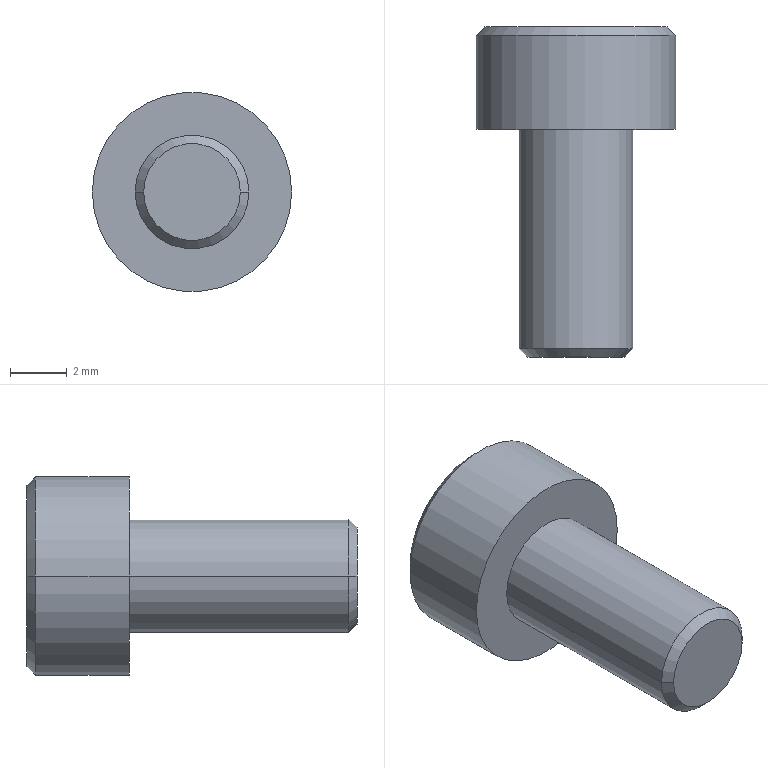Part | NX | 1 solid | 56 faces | box 7 x 11.6 x 7 mm | volume 221.628 mm3 | plane 44 | cone 6 | cylinder 6 | commonest cylinder face diameters 3 x2 4 x2 7 x2
STEP:
#1=CARTESIAN_POINT('',(-1.7,-8.,0.));
#2=VERTEX_POINT('',#1);
#3=CARTESIAN_POINT('',(1.7,-8.,0.));
#4=VERTEX_POINT('',#3);
#5=CARTESIAN_POINT('',(0.,-8.,0.));
#6=DIRECTION('',(0.,1.,0.));
#7=DIRECTION('',(-1.,0.,0.));
#8=AXIS2_PLACEMENT_3D('',#5,#6,#7);
#9=CIRCLE('',#8,1.7);
#10=EDGE_CURVE('',#2,#4,#9,.T.);
#11=ORIENTED_EDGE('',*,*,#10,.F.);
#12=CARTESIAN_POINT('',(0.,-8.,0.));
#13=DIRECTION('',(0.,1.,0.));
#14=DIRECTION('',(-1.,0.,0.));
#15=AXIS2_PLACEMENT_3D('',#12,#13,#14);
#16=CIRCLE('',#15,1.7);
#17=EDGE_CURVE('',#4,#2,#16,.T.);
#18=ORIENTED_EDGE('',*,*,#17,.F.);
#19=EDGE_LOOP('',(#11,#18));
#20=FACE_BOUND('',#19,.T.);
#21=CARTESIAN_POINT('',(0.,-8.,0.));
#22=DIRECTION('',(0.,-1.,0.));
#23=DIRECTION('',(0.,0.,-1.));
#24=AXIS2_PLACEMENT_3D('',#21,#22,#23);
#25=PLANE('',#24);
#26=ADVANCED_FACE('',(#20),#25,.T.);
#27=ORIENTED_EDGE('',*,*,#10,.T.);
#28=CARTESIAN_POINT('',(2.,-7.7,0.));
#29=VERTEX_POINT('',#28);
#30=CARTESIAN_POINT('',(1.85,-7.85,0.));
#31=DIRECTION('',(0.7071,0.7071,0.));
#32=VECTOR('',#31,1000.);
#33=LINE('',#30,#32);
#34=EDGE_CURVE('',#4,#29,#33,.T.);
#35=ORIENTED_EDGE('',*,*,#34,.T.);
#36=CARTESIAN_POINT('',(-2.,-7.7,0.));
#37=VERTEX_POINT('',#36);
#38=CARTESIAN_POINT('',(0.,-7.7,0.));
#39=DIRECTION('',(0.,1.,0.));
#40=DIRECTION('',(-1.,0.,0.));
#41=AXIS2_PLACEMENT_3D('',#38,#39,#40);
#42=CIRCLE('',#41,2.);
#43=EDGE_CURVE('',#37,#29,#42,.T.);
#44=ORIENTED_EDGE('',*,*,#43,.F.);
#45=CARTESIAN_POINT('',(-1.85,-7.85,0.));
#46=DIRECTION('',(-0.7071,0.7071,0.));
#47=VECTOR('',#46,1000.);
#48=LINE('',#45,#47);
#49=EDGE_CURVE('',#2,#37,#48,.T.);
#50=ORIENTED_EDGE('',*,*,#49,.F.);
#51=EDGE_LOOP('',(#27,#35,#44,#50));
#52=FACE_BOUND('',#51,.T.);
#53=CARTESIAN_POINT('',(0.,-7.85,0.));
#54=DIRECTION('',(0.,1.,0.));
#55=DIRECTION('',(1.,0.,0.));
#56=AXIS2_PLACEMENT_3D('',#53,#54,#55);
#57=CONICAL_SURFACE('',#56,1.85,0.7854);
#58=ADVANCED_FACE('',(#52),#57,.T.);
#59=CARTESIAN_POINT('',(0.,-7.7,0.));
#60=DIRECTION('',(0.,1.,0.));
#61=DIRECTION('',(-1.,0.,0.));
#62=AXIS2_PLACEMENT_3D('',#59,#60,#61);
#63=CIRCLE('',#62,2.);
#64=EDGE_CURVE('',#29,#37,#63,.T.);
#65=ORIENTED_EDGE('',*,*,#64,.T.);
#66=CARTESIAN_POINT('',(-2.,0.,0.));
#67=VERTEX_POINT('',#66);
#68=CARTESIAN_POINT('',(-2.,4.18,0.));
#69=DIRECTION('',(0.,-1.,0.));
#70=VECTOR('',#69,1000.);
#71=LINE('',#68,#70);
#72=EDGE_CURVE('',#37,#67,#71,.F.);
#73=ORIENTED_EDGE('',*,*,#72,.T.);
#74=CARTESIAN_POINT('',(2.,0.,0.));
#75=VERTEX_POINT('',#74);
#76=CARTESIAN_POINT('',(0.,0.,0.));
#77=DIRECTION('',(0.,-1.,0.));
#78=DIRECTION('',(1.,0.,0.));
#79=AXIS2_PLACEMENT_3D('',#76,#77,#78);
#80=CIRCLE('',#79,2.);
#81=EDGE_CURVE('',#67,#75,#80,.T.);
#82=ORIENTED_EDGE('',*,*,#81,.T.);
#83=CARTESIAN_POINT('',(2.,4.18,0.));
#84=DIRECTION('',(0.,-1.,0.));
#85=VECTOR('',#84,1000.);
#86=LINE('',#83,#85);
#87=EDGE_CURVE('',#29,#75,#86,.F.);
#88=ORIENTED_EDGE('',*,*,#87,.F.);
#89=EDGE_LOOP('',(#65,#73,#82,#88));
#90=FACE_BOUND('',#89,.T.);
#91=CARTESIAN_POINT('',(0.,4.18,0.));
#92=DIRECTION('',(0.,-1.,0.));
#93=DIRECTION('',(-1.,0.,0.));
#94=AXIS2_PLACEMENT_3D('',#91,#92,#93);
#95=CYLINDRICAL_SURFACE('',#94,2.);
#96=ADVANCED_FACE('',(#90),#95,.T.);
#97=CARTESIAN_POINT('',(0.1875,3.6,1.945));
#98=VERTEX_POINT('',#97);
#99=CARTESIAN_POINT('',(0.4,3.6,1.702));
#100=VERTEX_POINT('',#99);
#101=CARTESIAN_POINT('',(0.1875,3.6,1.945));
#102=DIRECTION('',(0.659,0.,-0.7522));
#103=VECTOR('',#102,1000.);
#104=LINE('',#101,#103);
#105=EDGE_CURVE('',#98,#100,#104,.T.);
#106=ORIENTED_EDGE('',*,*,#105,.F.);
#107=CARTESIAN_POINT('',(0.4,3.6,1.945));
#108=VERTEX_POINT('',#107);
#109=CARTESIAN_POINT('',(0.1875,3.6,1.945));
#110=DIRECTION('',(1.,0.,0.));
#111=VECTOR('',#110,1000.);
#112=LINE('',#109,#111);
#113=EDGE_CURVE('',#98,#108,#112,.T.);
#114=ORIENTED_EDGE('',*,*,#113,.T.);
#115=CARTESIAN_POINT('',(0.4,3.6,1.945));
#116=DIRECTION('',(0.,0.,-1.));
#117=VECTOR('',#116,1000.);
#118=LINE('',#115,#117);
#119=EDGE_CURVE('',#108,#100,#118,.T.);
#120=ORIENTED_EDGE('',*,*,#119,.T.);
#121=EDGE_LOOP('',(#106,#114,#120));
#122=FACE_BOUND('',#121,.T.);
#123=CARTESIAN_POINT('',(0.,3.6,0.));
#124=DIRECTION('',(0.,-1.,0.));
#125=DIRECTION('',(0.,0.,-1.));
#126=AXIS2_PLACEMENT_3D('',#123,#124,#125);
#127=PLANE('',#126);
#128=ADVANCED_FACE('',(#122),#127,.F.);
#129=CARTESIAN_POINT('',(0.1,3.55,1.945));
#130=VERTEX_POINT('',#129);
#131=CARTESIAN_POINT('',(0.4,3.55,1.6));
#132=VERTEX_POINT('',#131);
#133=CARTESIAN_POINT('',(0.1,3.55,1.945));
#134=DIRECTION('',(0.6565,0.,-0.7543));
#135=VECTOR('',#134,1000.);
#136=LINE('',#133,#135);
#137=EDGE_CURVE('',#130,#132,#136,.T.);
#138=ORIENTED_EDGE('',*,*,#137,.F.);
#139=CARTESIAN_POINT('',(0.1,3.55,2.021));
#140=VERTEX_POINT('',#139);
#141=CARTESIAN_POINT('',(0.1,3.55,2.021));
#142=DIRECTION('',(0.,0.,-1.));
#143=VECTOR('',#142,1000.);
#144=LINE('',#141,#143);
#145=EDGE_CURVE('',#140,#130,#144,.T.);
#146=ORIENTED_EDGE('',*,*,#145,.F.);
#147=CARTESIAN_POINT('',(0.4,3.55,2.021));
#148=VERTEX_POINT('',#147);
#149=CARTESIAN_POINT('',(0.4,3.55,2.021));
#150=DIRECTION('',(-1.,0.,0.));
#151=VECTOR('',#150,1000.);
#152=LINE('',#149,#151);
#153=EDGE_CURVE('',#148,#140,#152,.T.);
#154=ORIENTED_EDGE('',*,*,#153,.F.);
#155=CARTESIAN_POINT('',(0.4,3.55,2.2));
#156=VERTEX_POINT('',#155);
#157=CARTESIAN_POINT('',(0.4,3.55,2.2));
#158=DIRECTION('',(0.,0.,-1.));
#159=VECTOR('',#158,1000.);
#160=LINE('',#157,#159);
#161=EDGE_CURVE('',#156,#148,#160,.T.);
#162=ORIENTED_EDGE('',*,*,#161,.F.);
#163=CARTESIAN_POINT('',(0.475,3.55,2.2));
#164=VERTEX_POINT('',#163);
#165=CARTESIAN_POINT('',(0.475,3.55,2.2));
#166=DIRECTION('',(-1.,0.,0.));
#167=VECTOR('',#166,1000.);
#168=LINE('',#165,#167);
#169=EDGE_CURVE('',#164,#156,#168,.T.);
#170=ORIENTED_EDGE('',*,*,#169,.F.);
#171=CARTESIAN_POINT('',(0.475,3.55,2.021));
#172=VERTEX_POINT('',#171);
#173=CARTESIAN_POINT('',(0.475,3.55,2.021));
#174=DIRECTION('',(0.,0.,1.));
#175=VECTOR('',#174,1000.);
#176=LINE('',#173,#175);
#177=EDGE_CURVE('',#172,#164,#176,.T.);
#178=ORIENTED_EDGE('',*,*,#177,.F.);
#179=CARTESIAN_POINT('',(0.6,3.55,2.021));
#180=VERTEX_POINT('',#179);
#181=CARTESIAN_POINT('',(0.6,3.55,2.021));
#182=DIRECTION('',(-1.,0.,0.));
#183=VECTOR('',#182,1000.);
#184=LINE('',#181,#183);
#185=EDGE_CURVE('',#180,#172,#184,.T.);
#186=ORIENTED_EDGE('',*,*,#185,.F.);
#187=CARTESIAN_POINT('',(0.6,3.55,1.945));
#188=VERTEX_POINT('',#187);
#189=CARTESIAN_POINT('',(0.6,3.55,1.945));
#190=DIRECTION('',(0.,0.,1.));
#191=VECTOR('',#190,1000.);
#192=LINE('',#189,#191);
#193=EDGE_CURVE('',#188,#180,#192,.T.);
#194=ORIENTED_EDGE('',*,*,#193,.F.);
#195=CARTESIAN_POINT('',(0.475,3.55,1.945));
#196=VERTEX_POINT('',#195);
#197=CARTESIAN_POINT('',(0.475,3.55,1.945));
#198=DIRECTION('',(1.,0.,0.));
#199=VECTOR('',#198,1000.);
#200=LINE('',#197,#199);
#201=EDGE_CURVE('',#196,#188,#200,.T.);
#202=ORIENTED_EDGE('',*,*,#201,.F.);
#203=CARTESIAN_POINT('',(0.475,3.55,1.6));
#204=VERTEX_POINT('',#203);
#205=CARTESIAN_POINT('',(0.475,3.55,1.6));
#206=DIRECTION('',(0.,0.,1.));
#207=VECTOR('',#206,1000.);
#208=LINE('',#205,#207);
#209=EDGE_CURVE('',#204,#196,#208,.T.);
#210=ORIENTED_EDGE('',*,*,#209,.F.);
#211=CARTESIAN_POINT('',(0.4,3.55,1.6));
#212=DIRECTION('',(1.,0.,0.));
#213=VECTOR('',#212,1000.);
#214=LINE('',#211,#213);
#215=EDGE_CURVE('',#132,#204,#214,.T.);
#216=ORIENTED_EDGE('',*,*,#215,.F.);
#217=EDGE_LOOP('',(#138,#146,#154,#162,#170,#178,#186,#194,#202,#210,#216));
#218=FACE_BOUND('',#217,.T.);
#219=CARTESIAN_POINT('',(0.4,3.55,1.702));
#220=VERTEX_POINT('',#219);
#221=CARTESIAN_POINT('',(0.1875,3.55,1.945));
#222=VERTEX_POINT('',#221);
#223=CARTESIAN_POINT('',(0.4,3.55,1.702));
#224=DIRECTION('',(-0.659,0.,0.7522));
#225=VECTOR('',#224,1000.);
#226=LINE('',#223,#225);
#227=EDGE_CURVE('',#220,#222,#226,.T.);
#228=ORIENTED_EDGE('',*,*,#227,.F.);
#229=CARTESIAN_POINT('',(0.4,3.55,1.945));
#230=VERTEX_POINT('',#229);
#231=CARTESIAN_POINT('',(0.4,3.55,1.945));
#232=DIRECTION('',(0.,0.,-1.));
#233=VECTOR('',#232,1000.);
#234=LINE('',#231,#233);
#235=EDGE_CURVE('',#230,#220,#234,.T.);
#236=ORIENTED_EDGE('',*,*,#235,.F.);
#237=CARTESIAN_POINT('',(0.1875,3.55,1.945));
#238=DIRECTION('',(1.,0.,0.));
#239=VECTOR('',#238,1000.);
#240=LINE('',#237,#239);
#241=EDGE_CURVE('',#222,#230,#240,.T.);
#242=ORIENTED_EDGE('',*,*,#241,.F.);
#243=EDGE_LOOP('',(#228,#236,#242));
#244=FACE_BOUND('',#243,.T.);
#245=CARTESIAN_POINT('',(0.,3.55,0.));
#246=DIRECTION('',(0.,1.,0.));
#247=DIRECTION('',(1.,0.,0.));
#248=AXIS2_PLACEMENT_3D('',#245,#246,#247);
#249=PLANE('',#248);
#250=ADVANCED_FACE('',(#218,#244),#249,.T.);
#251=CARTESIAN_POINT('',(3.5,0.,0.));
#252=VERTEX_POINT('',#251);
#253=CARTESIAN_POINT('',(-3.5,0.,0.));
#254=VERTEX_POINT('',#253);
#255=CARTESIAN_POINT('',(0.,0.,0.));
#256=DIRECTION('',(0.,1.,0.));
#257=DIRECTION('',(-1.,0.,0.));
#258=AXIS2_PLACEMENT_3D('',#255,#256,#257);
#259=CIRCLE('',#258,3.5);
#260=EDGE_CURVE('',#252,#254,#259,.T.);
#261=ORIENTED_EDGE('',*,*,#260,.F.);
#262=CARTESIAN_POINT('',(0.,0.,0.));
#263=DIRECTION('',(0.,1.,0.));
#264=DIRECTION('',(-1.,0.,0.));
#265=AXIS2_PLACEMENT_3D('',#262,#263,#264);
#266=CIRCLE('',#265,3.5);
#267=EDGE_CURVE('',#254,#252,#266,.T.);
#268=ORIENTED_EDGE('',*,*,#267,.F.);
#269=EDGE_LOOP('',(#261,#268));
#270=FACE_BOUND('',#269,.T.);
#271=ORIENTED_EDGE('',*,*,#81,.F.);
#272=CARTESIAN_POINT('',(0.,0.,0.));
#273=DIRECTION('',(0.,-1.,0.));
#274=DIRECTION('',(1.,0.,0.));
#275=AXIS2_PLACEMENT_3D('',#272,#273,#274);
#276=CIRCLE('',#275,2.);
#277=EDGE_CURVE('',#75,#67,#276,.T.);
#278=ORIENTED_EDGE('',*,*,#277,.F.);
#279=EDGE_LOOP('',(#271,#278));
#280=FACE_BOUND('',#279,.T.);
#281=CARTESIAN_POINT('',(0.,0.,0.));
#282=DIRECTION('',(0.,-1.,0.));
#283=DIRECTION('',(0.,0.,-1.));
#284=AXIS2_PLACEMENT_3D('',#281,#282,#283);
#285=PLANE('',#284);
#286=ADVANCED_FACE('',(#270,#280),#285,.T.);
#287=CARTESIAN_POINT('',(-3.5,3.3,0.));
#288=VERTEX_POINT('',#287);
#289=CARTESIAN_POINT('',(3.5,3.3,0.));
#290=VERTEX_POINT('',#289);
#291=CARTESIAN_POINT('',(0.,3.3,0.));
#292=DIRECTION('',(0.,-1.,0.));
#293=DIRECTION('',(-1.,0.,0.));
#294=AXIS2_PLACEMENT_3D('',#291,#292,#293);
#295=CIRCLE('',#294,3.5);
#296=EDGE_CURVE('',#288,#290,#295,.T.);
#297=ORIENTED_EDGE('',*,*,#296,.T.);
#298=CARTESIAN_POINT('',(3.5,4.18,0.));
#299=DIRECTION('',(0.,-1.,0.));
#300=VECTOR('',#299,1000.);
#301=LINE('',#298,#300);
#302=EDGE_CURVE('',#252,#290,#301,.F.);
#303=ORIENTED_EDGE('',*,*,#302,.F.);
#304=ORIENTED_EDGE('',*,*,#260,.T.);
#305=CARTESIAN_POINT('',(-3.5,4.18,0.));
#306=DIRECTION('',(0.,-1.,0.));
#307=VECTOR('',#306,1000.);
#308=LINE('',#305,#307);
#309=EDGE_CURVE('',#254,#288,#308,.F.);
#310=ORIENTED_EDGE('',*,*,#309,.T.);
#311=EDGE_LOOP('',(#297,#303,#304,#310));
#312=FACE_BOUND('',#311,.T.);
#313=CARTESIAN_POINT('',(0.,4.18,0.));
#314=DIRECTION('',(0.,-1.,0.));
#315=DIRECTION('',(-1.,0.,0.));
#316=AXIS2_PLACEMENT_3D('',#313,#314,#315);
#317=CYLINDRICAL_SURFACE('',#316,3.5);
#318=ADVANCED_FACE('',(#312),#317,.T.);
#319=ORIENTED_EDGE('',*,*,#105,.T.);
#320=CARTESIAN_POINT('',(0.4,3.55,1.702));
#321=DIRECTION('',(0.,1.,0.));
#322=VECTOR('',#321,1000.);
#323=LINE('',#320,#322);
#324=EDGE_CURVE('',#220,#100,#323,.T.);
#325=ORIENTED_EDGE('',*,*,#324,.F.);
#326=ORIENTED_EDGE('',*,*,#227,.T.);
#327=CARTESIAN_POINT('',(0.1875,3.55,1.945));
#328=DIRECTION('',(0.,1.,0.));
#329=VECTOR('',#328,1000.);
#330=LINE('',#327,#329);
#331=EDGE_CURVE('',#222,#98,#330,.T.);
#332=ORIENTED_EDGE('',*,*,#331,.T.);
#333=EDGE_LOOP('',(#319,#325,#326,#332));
#334=FACE_BOUND('',#333,.T.);
#335=CARTESIAN_POINT('',(0.1875,3.6,1.945));
#336=DIRECTION('',(0.7522,0.,0.659));
#337=DIRECTION('',(0.,-1.,0.));
#338=AXIS2_PLACEMENT_3D('',#335,#336,#337);
#339=PLANE('',#338);
#340=ADVANCED_FACE('',(#334),#339,.F.);
#341=CARTESIAN_POINT('',(3.2,3.6,0.));
#342=VERTEX_POINT('',#341);
#343=CARTESIAN_POINT('',(-3.2,3.6,0.));
#344=VERTEX_POINT('',#343);
#345=CARTESIAN_POINT('',(0.,3.6,0.));
#346=DIRECTION('',(0.,-1.,0.));
#347=DIRECTION('',(-1.,0.,0.));
#348=AXIS2_PLACEMENT_3D('',#345,#346,#347);
#349=CIRCLE('',#348,3.2);
#350=EDGE_CURVE('',#342,#344,#349,.T.);
#351=ORIENTED_EDGE('',*,*,#350,.T.);
#352=CARTESIAN_POINT('',(-3.35,3.45,0.));
#353=DIRECTION('',(-0.7071,-0.7071,0.));
#354=VECTOR('',#353,1000.);
#355=LINE('',#352,#354);
#356=EDGE_CURVE('',#288,#344,#355,.F.);
#357=ORIENTED_EDGE('',*,*,#356,.F.);
#358=CARTESIAN_POINT('',(0.,3.3,0.));
#359=DIRECTION('',(0.,-1.,0.));
#360=DIRECTION('',(-1.,0.,0.));
#361=AXIS2_PLACEMENT_3D('',#358,#359,#360);
#362=CIRCLE('',#361,3.5);
#363=EDGE_CURVE('',#290,#288,#362,.T.);
#364=ORIENTED_EDGE('',*,*,#363,.F.);
#365=CARTESIAN_POINT('',(3.35,3.45,0.));
#366=DIRECTION('',(0.7071,-0.7071,0.));
#367=VECTOR('',#366,1000.);
#368=LINE('',#365,#367);
#369=EDGE_CURVE('',#290,#342,#368,.F.);
#370=ORIENTED_EDGE('',*,*,#369,.T.);
#371=EDGE_LOOP('',(#351,#357,#364,#370));
#372=FACE_BOUND('',#371,.T.);
#373=CARTESIAN_POINT('',(0.,3.45,0.));
#374=DIRECTION('',(0.,-1.,0.));
#375=DIRECTION('',(-1.,0.,0.));
#376=AXIS2_PLACEMENT_3D('',#373,#374,#375);
#377=CONICAL_SURFACE('',#376,3.35,0.7854);
#378=ADVANCED_FACE('',(#372),#377,.T.);
#379=ORIENTED_EDGE('',*,*,#350,.F.);
#380=CARTESIAN_POINT('',(0.,3.6,0.));
#381=DIRECTION('',(0.,-1.,0.));
#382=DIRECTION('',(-1.,0.,0.));
#383=AXIS2_PLACEMENT_3D('',#380,#381,#382);
#384=CIRCLE('',#383,3.2);
#385=EDGE_CURVE('',#344,#342,#384,.T.);
#386=ORIENTED_EDGE('',*,*,#385,.F.);
#387=EDGE_LOOP('',(#379,#386));
#388=FACE_BOUND('',#387,.T.);
#389=CARTESIAN_POINT('',(-0.075,3.6,2.2));
#390=VERTEX_POINT('',#389);
#391=CARTESIAN_POINT('',(-0.075,3.6,1.728));
#392=VERTEX_POINT('',#391);
#393=CARTESIAN_POINT('',(-0.075,3.6,2.2));
#394=DIRECTION('',(0.,0.,-1.));
#395=VECTOR('',#394,1000.);
#396=LINE('',#393,#395);
#397=EDGE_CURVE('',#390,#392,#396,.T.);
#398=ORIENTED_EDGE('',*,*,#397,.T.);
#399=CARTESIAN_POINT('',(-0.25,3.6,2.2));
#400=VERTEX_POINT('',#399);
#401=CARTESIAN_POINT('',(-0.25,3.6,2.2));
#402=DIRECTION('',(0.3474,0.,-0.9377));
#403=VECTOR('',#402,1000.);
#404=LINE('',#401,#403);
#405=EDGE_CURVE('',#400,#392,#404,.T.);
#406=ORIENTED_EDGE('',*,*,#405,.F.);
#407=CARTESIAN_POINT('',(-0.35,3.6,2.2));
#408=VERTEX_POINT('',#407);
#409=CARTESIAN_POINT('',(-0.25,3.6,2.2));
#410=DIRECTION('',(-1.,0.,0.));
#411=VECTOR('',#410,1000.);
#412=LINE('',#409,#411);
#413=EDGE_CURVE('',#400,#408,#412,.T.);
#414=ORIENTED_EDGE('',*,*,#413,.T.);
#415=CARTESIAN_POINT('',(-0.525,3.6,1.728));
#416=VERTEX_POINT('',#415);
#417=CARTESIAN_POINT('',(-0.525,3.6,1.728));
#418=DIRECTION('',(0.3474,0.,0.9377));
#419=VECTOR('',#418,1000.);
#420=LINE('',#417,#419);
#421=EDGE_CURVE('',#416,#408,#420,.T.);
#422=ORIENTED_EDGE('',*,*,#421,.F.);
#423=CARTESIAN_POINT('',(-0.525,3.6,2.2));
#424=VERTEX_POINT('',#423);
#425=CARTESIAN_POINT('',(-0.525,3.6,1.728));
#426=DIRECTION('',(0.,0.,1.));
#427=VECTOR('',#426,1000.);
#428=LINE('',#425,#427);
#429=EDGE_CURVE('',#416,#424,#428,.T.);
#430=ORIENTED_EDGE('',*,*,#429,.T.);
#431=CARTESIAN_POINT('',(-0.6,3.6,2.2));
#432=VERTEX_POINT('',#431);
#433=CARTESIAN_POINT('',(-0.525,3.6,2.2));
#434=DIRECTION('',(-1.,0.,0.));
#435=VECTOR('',#434,1000.);
#436=LINE('',#433,#435);
#437=EDGE_CURVE('',#424,#432,#436,.T.);
#438=ORIENTED_EDGE('',*,*,#437,.T.);
#439=CARTESIAN_POINT('',(-0.6,3.6,1.6));
#440=VERTEX_POINT('',#439);
#441=CARTESIAN_POINT('',(-0.6,3.6,2.2));
#442=DIRECTION('',(0.,0.,-1.));
#443=VECTOR('',#442,1000.);
#444=LINE('',#441,#443);
#445=EDGE_CURVE('',#432,#440,#444,.T.);
#446=ORIENTED_EDGE('',*,*,#445,.T.);
#447=CARTESIAN_POINT('',(-0.4875,3.6,1.6));
#448=VERTEX_POINT('',#447);
#449=CARTESIAN_POINT('',(-0.6,3.6,1.6));
#450=DIRECTION('',(1.,0.,0.));
#451=VECTOR('',#450,1000.);
#452=LINE('',#449,#451);
#453=EDGE_CURVE('',#440,#448,#452,.T.);
#454=ORIENTED_EDGE('',*,*,#453,.T.);
#455=CARTESIAN_POINT('',(-0.3,3.6,2.136));
#456=VERTEX_POINT('',#455);
#457=CARTESIAN_POINT('',(-0.3,3.6,2.136));
#458=DIRECTION('',(-0.3301,0.,-0.9439));
#459=VECTOR('',#458,1000.);
#460=LINE('',#457,#459);
#461=EDGE_CURVE('',#456,#448,#460,.T.);
#462=ORIENTED_EDGE('',*,*,#461,.F.);
#463=CARTESIAN_POINT('',(-0.132,3.6,1.656));
#464=VERTEX_POINT('',#463);
#465=CARTESIAN_POINT('',(-0.132,3.6,1.656));
#466=DIRECTION('',(-0.3301,0.,0.9439));
#467=VECTOR('',#466,1000.);
#468=LINE('',#465,#467);
#469=EDGE_CURVE('',#464,#456,#468,.T.);
#470=ORIENTED_EDGE('',*,*,#469,.F.);
#471=CARTESIAN_POINT('',(-1.5,3.6,0.866));
#472=VERTEX_POINT('',#471);
#473=CARTESIAN_POINT('',(-1.5,3.6,0.866));
#474=DIRECTION('',(0.866,0.,0.5));
#475=VECTOR('',#474,1000.);
#476=LINE('',#473,#475);
#477=EDGE_CURVE('',#472,#464,#476,.T.);
#478=ORIENTED_EDGE('',*,*,#477,.F.);
#479=CARTESIAN_POINT('',(-1.5,3.6,-0.866));
#480=VERTEX_POINT('',#479);
#481=CARTESIAN_POINT('',(-1.5,3.6,0.866));
#482=DIRECTION('',(0.,0.,-1.));
#483=VECTOR('',#482,1000.);
#484=LINE('',#481,#483);
#485=EDGE_CURVE('',#472,#480,#484,.T.);
#486=ORIENTED_EDGE('',*,*,#485,.T.);
#487=CARTESIAN_POINT('',(0.,3.6,-1.732));
#488=VERTEX_POINT('',#487);
#489=CARTESIAN_POINT('',(0.,3.6,-1.732));
#490=DIRECTION('',(-0.866,0.,0.5));
#491=VECTOR('',#490,1000.);
#492=LINE('',#489,#491);
#493=EDGE_CURVE('',#488,#480,#492,.T.);
#494=ORIENTED_EDGE('',*,*,#493,.F.);
#495=CARTESIAN_POINT('',(1.5,3.6,-0.866));
#496=VERTEX_POINT('',#495);
#497=CARTESIAN_POINT('',(1.5,3.6,-0.866));
#498=DIRECTION('',(-0.866,0.,-0.5));
#499=VECTOR('',#498,1000.);
#500=LINE('',#497,#499);
#501=EDGE_CURVE('',#496,#488,#500,.T.);
#502=ORIENTED_EDGE('',*,*,#501,.F.);
#503=CARTESIAN_POINT('',(1.5,3.6,0.866));
#504=VERTEX_POINT('',#503);
#505=CARTESIAN_POINT('',(1.5,3.6,-0.866));
#506=DIRECTION('',(0.,0.,1.));
#507=VECTOR('',#506,1000.);
#508=LINE('',#505,#507);
#509=EDGE_CURVE('',#496,#504,#508,.T.);
#510=ORIENTED_EDGE('',*,*,#509,.T.);
#511=CARTESIAN_POINT('',(0.,3.6,1.732));
#512=VERTEX_POINT('',#511);
#513=CARTESIAN_POINT('',(0.,3.6,1.732));
#514=DIRECTION('',(0.866,0.,-0.5));
#515=VECTOR('',#514,1000.);
#516=LINE('',#513,#515);
#517=EDGE_CURVE('',#512,#504,#516,.T.);
#518=ORIENTED_EDGE('',*,*,#517,.F.);
#519=CARTESIAN_POINT('',(0.,3.6,2.2));
#520=VERTEX_POINT('',#519);
#521=CARTESIAN_POINT('',(0.,3.6,1.732));
#522=DIRECTION('',(0.,0.,1.));
#523=VECTOR('',#522,1000.);
#524=LINE('',#521,#523);
#525=EDGE_CURVE('',#512,#520,#524,.T.);
#526=ORIENTED_EDGE('',*,*,#525,.T.);
#527=CARTESIAN_POINT('',(0.,3.6,2.2));
#528=DIRECTION('',(-1.,0.,0.));
#529=VECTOR('',#528,1000.);
#530=LINE('',#527,#529);
#531=EDGE_CURVE('',#520,#390,#530,.T.);
#532=ORIENTED_EDGE('',*,*,#531,.T.);
#533=EDGE_LOOP('',(#398,#406,#414,#422,#430,#438,#446,#454,#462,#470,#478,#486,#494,#502,#510,#518,#526,#532));
#534=FACE_BOUND('',#533,.T.);
#535=CARTESIAN_POINT('',(0.4,3.6,1.6));
#536=VERTEX_POINT('',#535);
#537=CARTESIAN_POINT('',(0.1,3.6,1.945));
#538=VERTEX_POINT('',#537);
#539=CARTESIAN_POINT('',(0.4,3.6,1.6));
#540=DIRECTION('',(-0.6565,0.,0.7543));
#541=VECTOR('',#540,1000.);
#542=LINE('',#539,#541);
#543=EDGE_CURVE('',#536,#538,#542,.T.);
#544=ORIENTED_EDGE('',*,*,#543,.F.);
#545=CARTESIAN_POINT('',(0.475,3.6,1.6));
#546=VERTEX_POINT('',#545);
#547=CARTESIAN_POINT('',(0.4,3.6,1.6));
#548=DIRECTION('',(1.,0.,0.));
#549=VECTOR('',#548,1000.);
#550=LINE('',#547,#549);
#551=EDGE_CURVE('',#536,#546,#550,.T.);
#552=ORIENTED_EDGE('',*,*,#551,.T.);
#553=CARTESIAN_POINT('',(0.475,3.6,1.945));
#554=VERTEX_POINT('',#553);
#555=CARTESIAN_POINT('',(0.475,3.6,1.6));
#556=DIRECTION('',(0.,0.,1.));
#557=VECTOR('',#556,1000.);
#558=LINE('',#555,#557);
#559=EDGE_CURVE('',#546,#554,#558,.T.);
#560=ORIENTED_EDGE('',*,*,#559,.T.);
#561=CARTESIAN_POINT('',(0.6,3.6,1.945));
#562=VERTEX_POINT('',#561);
#563=CARTESIAN_POINT('',(0.475,3.6,1.945));
#564=DIRECTION('',(1.,0.,0.));
#565=VECTOR('',#564,1000.);
#566=LINE('',#563,#565);
#567=EDGE_CURVE('',#554,#562,#566,.T.);
#568=ORIENTED_EDGE('',*,*,#567,.T.);
#569=CARTESIAN_POINT('',(0.6,3.6,2.021));
#570=VERTEX_POINT('',#569);
#571=CARTESIAN_POINT('',(0.6,3.6,1.945));
#572=DIRECTION('',(0.,0.,1.));
#573=VECTOR('',#572,1000.);
#574=LINE('',#571,#573);
#575=EDGE_CURVE('',#562,#570,#574,.T.);
#576=ORIENTED_EDGE('',*,*,#575,.T.);
#577=CARTESIAN_POINT('',(0.475,3.6,2.021));
#578=VERTEX_POINT('',#577);
#579=CARTESIAN_POINT('',(0.6,3.6,2.021));
#580=DIRECTION('',(-1.,0.,0.));
#581=VECTOR('',#580,1000.);
#582=LINE('',#579,#581);
#583=EDGE_CURVE('',#570,#578,#582,.T.);
#584=ORIENTED_EDGE('',*,*,#583,.T.);
#585=CARTESIAN_POINT('',(0.475,3.6,2.2));
#586=VERTEX_POINT('',#585);
#587=CARTESIAN_POINT('',(0.475,3.6,2.021));
#588=DIRECTION('',(0.,0.,1.));
#589=VECTOR('',#588,1000.);
#590=LINE('',#587,#589);
#591=EDGE_CURVE('',#578,#586,#590,.T.);
#592=ORIENTED_EDGE('',*,*,#591,.T.);
#593=CARTESIAN_POINT('',(0.4,3.6,2.2));
#594=VERTEX_POINT('',#593);
#595=CARTESIAN_POINT('',(0.475,3.6,2.2));
#596=DIRECTION('',(-1.,0.,0.));
#597=VECTOR('',#596,1000.);
#598=LINE('',#595,#597);
#599=EDGE_CURVE('',#586,#594,#598,.T.);
#600=ORIENTED_EDGE('',*,*,#599,.T.);
#601=CARTESIAN_POINT('',(0.4,3.6,2.021));
#602=VERTEX_POINT('',#601);
#603=CARTESIAN_POINT('',(0.4,3.6,2.2));
#604=DIRECTION('',(0.,0.,-1.));
#605=VECTOR('',#604,1000.);
#606=LINE('',#603,#605);
#607=EDGE_CURVE('',#594,#602,#606,.T.);
#608=ORIENTED_EDGE('',*,*,#607,.T.);
#609=CARTESIAN_POINT('',(0.1,3.6,2.021));
#610=VERTEX_POINT('',#609);
#611=CARTESIAN_POINT('',(0.4,3.6,2.021));
#612=DIRECTION('',(-1.,0.,0.));
#613=VECTOR('',#612,1000.);
#614=LINE('',#611,#613);
#615=EDGE_CURVE('',#602,#610,#614,.T.);
#616=ORIENTED_EDGE('',*,*,#615,.T.);
#617=CARTESIAN_POINT('',(0.1,3.6,2.021));
#618=DIRECTION('',(0.,0.,-1.));
#619=VECTOR('',#618,1000.);
#620=LINE('',#617,#619);
#621=EDGE_CURVE('',#610,#538,#620,.T.);
#622=ORIENTED_EDGE('',*,*,#621,.T.);
#623=EDGE_LOOP('',(#544,#552,#560,#568,#576,#584,#592,#600,#608,#616,#622));
#624=FACE_BOUND('',#623,.T.);
#625=CARTESIAN_POINT('',(0.,3.6,0.));
#626=DIRECTION('',(0.,-1.,0.));
#627=DIRECTION('',(0.,0.,-1.));
#628=AXIS2_PLACEMENT_3D('',#625,#626,#627);
#629=PLANE('',#628);
#630=ADVANCED_FACE('',(#388,#534,#624),#629,.F.);
#631=ORIENTED_EDGE('',*,*,#113,.F.);
#632=ORIENTED_EDGE('',*,*,#331,.F.);
#633=ORIENTED_EDGE('',*,*,#241,.T.);
#634=CARTESIAN_POINT('',(0.4,3.55,1.945));
#635=DIRECTION('',(0.,1.,0.));
#636=VECTOR('',#635,1000.);
#637=LINE('',#634,#636);
#638=EDGE_CURVE('',#230,#108,#637,.T.);
#639=ORIENTED_EDGE('',*,*,#638,.T.);
#640=EDGE_LOOP('',(#631,#632,#633,#639));
#641=FACE_BOUND('',#640,.T.);
#642=CARTESIAN_POINT('',(0.4,3.6,1.945));
#643=DIRECTION('',(0.,0.,-1.));
#644=DIRECTION('',(0.,-1.,0.));
#645=AXIS2_PLACEMENT_3D('',#642,#643,#644);
#646=PLANE('',#645);
#647=ADVANCED_FACE('',(#641),#646,.F.);
#648=ORIENTED_EDGE('',*,*,#397,.F.);
#649=CARTESIAN_POINT('',(-0.075,3.55,2.2));
#650=VERTEX_POINT('',#649);
#651=CARTESIAN_POINT('',(-0.075,3.55,2.2));
#652=DIRECTION('',(0.,1.,0.));
#653=VECTOR('',#652,1000.);
#654=LINE('',#651,#653);
#655=EDGE_CURVE('',#650,#390,#654,.T.);
#656=ORIENTED_EDGE('',*,*,#655,.F.);
#657=CARTESIAN_POINT('',(-0.075,3.55,1.728));
#658=VERTEX_POINT('',#657);
#659=CARTESIAN_POINT('',(-0.075,3.55,2.2));
#660=DIRECTION('',(0.,0.,-1.));
#661=VECTOR('',#660,1000.);
#662=LINE('',#659,#661);
#663=EDGE_CURVE('',#650,#658,#662,.T.);
#664=ORIENTED_EDGE('',*,*,#663,.T.);
#665=CARTESIAN_POINT('',(-0.075,3.55,1.728));
#666=DIRECTION('',(0.,1.,0.));
#667=VECTOR('',#666,1000.);
#668=LINE('',#665,#667);
#669=EDGE_CURVE('',#658,#392,#668,.T.);
#670=ORIENTED_EDGE('',*,*,#669,.T.);
#671=EDGE_LOOP('',(#648,#656,#664,#670));
#672=FACE_BOUND('',#671,.T.);
#673=CARTESIAN_POINT('',(-0.075,3.6,1.728));
#674=DIRECTION('',(-1.,0.,0.));
#675=DIRECTION('',(0.,0.,1.));
#676=AXIS2_PLACEMENT_3D('',#673,#674,#675);
#677=PLANE('',#676);
#678=ADVANCED_FACE('',(#672),#677,.F.);
#679=ORIENTED_EDGE('',*,*,#405,.T.);
#680=ORIENTED_EDGE('',*,*,#669,.F.);
#681=CARTESIAN_POINT('',(-0.25,3.55,2.2));
#682=VERTEX_POINT('',#681);
#683=CARTESIAN_POINT('',(-0.075,3.55,1.728));
#684=DIRECTION('',(-0.3474,0.,0.9377));
#685=VECTOR('',#684,1000.);
#686=LINE('',#683,#685);
#687=EDGE_CURVE('',#658,#682,#686,.T.);
#688=ORIENTED_EDGE('',*,*,#687,.T.);
#689=CARTESIAN_POINT('',(-0.25,3.55,2.2));
#690=DIRECTION('',(0.,1.,0.));
#691=VECTOR('',#690,1000.);
#692=LINE('',#689,#691);
#693=EDGE_CURVE('',#682,#400,#692,.T.);
#694=ORIENTED_EDGE('',*,*,#693,.T.);
#695=EDGE_LOOP('',(#679,#680,#688,#694));
#696=FACE_BOUND('',#695,.T.);
#697=CARTESIAN_POINT('',(-0.25,3.6,2.2));
#698=DIRECTION('',(0.9377,0.,0.3474));
#699=DIRECTION('',(0.,-1.,0.));
#700=AXIS2_PLACEMENT_3D('',#697,#698,#699);
#701=PLANE('',#700);
#702=ADVANCED_FACE('',(#696),#701,.F.);
#703=ORIENTED_EDGE('',*,*,#413,.F.);
#704=ORIENTED_EDGE('',*,*,#693,.F.);
#705=CARTESIAN_POINT('',(-0.35,3.55,2.2));
#706=VERTEX_POINT('',#705);
#707=CARTESIAN_POINT('',(-0.25,3.55,2.2));
#708=DIRECTION('',(-1.,0.,0.));
#709=VECTOR('',#708,1000.);
#710=LINE('',#707,#709);
#711=EDGE_CURVE('',#682,#706,#710,.T.);
#712=ORIENTED_EDGE('',*,*,#711,.T.);
#713=CARTESIAN_POINT('',(-0.35,3.55,2.2));
#714=DIRECTION('',(0.,1.,0.));
#715=VECTOR('',#714,1000.);
#716=LINE('',#713,#715);
#717=EDGE_CURVE('',#706,#408,#716,.T.);
#718=ORIENTED_EDGE('',*,*,#717,.T.);
#719=EDGE_LOOP('',(#703,#704,#712,#718));
#720=FACE_BOUND('',#719,.T.);
#721=CARTESIAN_POINT('',(-0.35,3.6,2.2));
#722=DIRECTION('',(0.,0.,1.));
#723=DIRECTION('',(1.,0.,0.));
#724=AXIS2_PLACEMENT_3D('',#721,#722,#723);
#725=PLANE('',#724);
#726=ADVANCED_FACE('',(#720),#725,.F.);
#727=ORIENTED_EDGE('',*,*,#421,.T.);
#728=ORIENTED_EDGE('',*,*,#717,.F.);
#729=CARTESIAN_POINT('',(-0.525,3.55,1.728));
#730=VERTEX_POINT('',#729);
#731=CARTESIAN_POINT('',(-0.35,3.55,2.2));
#732=DIRECTION('',(-0.3474,0.,-0.9377));
#733=VECTOR('',#732,1000.);
#734=LINE('',#731,#733);
#735=EDGE_CURVE('',#706,#730,#734,.T.);
#736=ORIENTED_EDGE('',*,*,#735,.T.);
#737=CARTESIAN_POINT('',(-0.525,3.55,1.728));
#738=DIRECTION('',(0.,1.,0.));
#739=VECTOR('',#738,1000.);
#740=LINE('',#737,#739);
#741=EDGE_CURVE('',#730,#416,#740,.T.);
#742=ORIENTED_EDGE('',*,*,#741,.T.);
#743=EDGE_LOOP('',(#727,#728,#736,#742));
#744=FACE_BOUND('',#743,.T.);
#745=CARTESIAN_POINT('',(-0.525,3.6,1.728));
#746=DIRECTION('',(-0.9377,0.,0.3474));
#747=DIRECTION('',(0.,1.,0.));
#748=AXIS2_PLACEMENT_3D('',#745,#746,#747);
#749=PLANE('',#748);
#750=ADVANCED_FACE('',(#744),#749,.F.);
#751=ORIENTED_EDGE('',*,*,#429,.F.);
#752=ORIENTED_EDGE('',*,*,#741,.F.);
#753=CARTESIAN_POINT('',(-0.525,3.55,2.2));
#754=VERTEX_POINT('',#753);
#755=CARTESIAN_POINT('',(-0.525,3.55,1.728));
#756=DIRECTION('',(0.,0.,1.));
#757=VECTOR('',#756,1000.);
#758=LINE('',#755,#757);
#759=EDGE_CURVE('',#730,#754,#758,.T.);
#760=ORIENTED_EDGE('',*,*,#759,.T.);
#761=CARTESIAN_POINT('',(-0.525,3.55,2.2));
#762=DIRECTION('',(0.,1.,0.));
#763=VECTOR('',#762,1000.);
#764=LINE('',#761,#763);
#765=EDGE_CURVE('',#754,#424,#764,.T.);
#766=ORIENTED_EDGE('',*,*,#765,.T.);
#767=EDGE_LOOP('',(#751,#752,#760,#766));
#768=FACE_BOUND('',#767,.T.);
#769=CARTESIAN_POINT('',(-0.525,3.6,2.2));
#770=DIRECTION('',(1.,0.,0.));
#771=DIRECTION('',(0.,1.,0.));
#772=AXIS2_PLACEMENT_3D('',#769,#770,#771);
#773=PLANE('',#772);
#774=ADVANCED_FACE('',(#768),#773,.F.);
#775=ORIENTED_EDGE('',*,*,#437,.F.);
#776=ORIENTED_EDGE('',*,*,#765,.F.);
#777=CARTESIAN_POINT('',(-0.6,3.55,2.2));
#778=VERTEX_POINT('',#777);
#779=CARTESIAN_POINT('',(-0.525,3.55,2.2));
#780=DIRECTION('',(-1.,0.,0.));
#781=VECTOR('',#780,1000.);
#782=LINE('',#779,#781);
#783=EDGE_CURVE('',#754,#778,#782,.T.);
#784=ORIENTED_EDGE('',*,*,#783,.T.);
#785=CARTESIAN_POINT('',(-0.6,3.55,2.2));
#786=DIRECTION('',(0.,1.,0.));
#787=VECTOR('',#786,1000.);
#788=LINE('',#785,#787);
#789=EDGE_CURVE('',#778,#432,#788,.T.);
#790=ORIENTED_EDGE('',*,*,#789,.T.);
#791=EDGE_LOOP('',(#775,#776,#784,#790));
#792=FACE_BOUND('',#791,.T.);
#793=CARTESIAN_POINT('',(-0.6,3.6,2.2));
#794=DIRECTION('',(0.,0.,1.));
#795=DIRECTION('',(1.,0.,0.));
#796=AXIS2_PLACEMENT_3D('',#793,#794,#795);
#797=PLANE('',#796);
#798=ADVANCED_FACE('',(#792),#797,.F.);
#799=ORIENTED_EDGE('',*,*,#445,.F.);
#800=ORIENTED_EDGE('',*,*,#789,.F.);
#801=CARTESIAN_POINT('',(-0.6,3.55,1.6));
#802=VERTEX_POINT('',#801);
#803=CARTESIAN_POINT('',(-0.6,3.55,2.2));
#804=DIRECTION('',(0.,0.,-1.));
#805=VECTOR('',#804,1000.);
#806=LINE('',#803,#805);
#807=EDGE_CURVE('',#778,#802,#806,.T.);
#808=ORIENTED_EDGE('',*,*,#807,.T.);
#809=CARTESIAN_POINT('',(-0.6,3.55,1.6));
#810=DIRECTION('',(0.,1.,0.));
#811=VECTOR('',#810,1000.);
#812=LINE('',#809,#811);
#813=EDGE_CURVE('',#802,#440,#812,.T.);
#814=ORIENTED_EDGE('',*,*,#813,.T.);
#815=EDGE_LOOP('',(#799,#800,#808,#814));
#816=FACE_BOUND('',#815,.T.);
#817=CARTESIAN_POINT('',(-0.6,3.6,1.6));
#818=DIRECTION('',(-1.,0.,0.));
#819=DIRECTION('',(0.,0.,1.));
#820=AXIS2_PLACEMENT_3D('',#817,#818,#819);
#821=PLANE('',#820);
#822=ADVANCED_FACE('',(#816),#821,.F.);
#823=ORIENTED_EDGE('',*,*,#453,.F.);
#824=ORIENTED_EDGE('',*,*,#813,.F.);
#825=CARTESIAN_POINT('',(-0.4875,3.55,1.6));
#826=VERTEX_POINT('',#825);
#827=CARTESIAN_POINT('',(-0.6,3.55,1.6));
#828=DIRECTION('',(1.,0.,0.));
#829=VECTOR('',#828,1000.);
#830=LINE('',#827,#829);
#831=EDGE_CURVE('',#802,#826,#830,.T.);
#832=ORIENTED_EDGE('',*,*,#831,.T.);
#833=CARTESIAN_POINT('',(-0.4875,3.55,1.6));
#834=DIRECTION('',(0.,1.,0.));
#835=VECTOR('',#834,1000.);
#836=LINE('',#833,#835);
#837=EDGE_CURVE('',#826,#448,#836,.T.);
#838=ORIENTED_EDGE('',*,*,#837,.T.);
#839=EDGE_LOOP('',(#823,#824,#832,#838));
#840=FACE_BOUND('',#839,.T.);
#841=CARTESIAN_POINT('',(-0.4875,3.6,1.6));
#842=DIRECTION('',(0.,0.,-1.));
#843=DIRECTION('',(0.,-1.,0.));
#844=AXIS2_PLACEMENT_3D('',#841,#842,#843);
#845=PLANE('',#844);
#846=ADVANCED_FACE('',(#840),#845,.F.);
#847=ORIENTED_EDGE('',*,*,#461,.T.);
#848=ORIENTED_EDGE('',*,*,#837,.F.);
#849=CARTESIAN_POINT('',(-0.3,3.55,2.136));
#850=VERTEX_POINT('',#849);
#851=CARTESIAN_POINT('',(-0.4875,3.55,1.6));
#852=DIRECTION('',(0.3301,0.,0.9439));
#853=VECTOR('',#852,1000.);
#854=LINE('',#851,#853);
#855=EDGE_CURVE('',#826,#850,#854,.T.);
#856=ORIENTED_EDGE('',*,*,#855,.T.);
#857=CARTESIAN_POINT('',(-0.3,3.55,2.136));
#858=DIRECTION('',(0.,1.,0.));
#859=VECTOR('',#858,1000.);
#860=LINE('',#857,#859);
#861=EDGE_CURVE('',#850,#456,#860,.T.);
#862=ORIENTED_EDGE('',*,*,#861,.T.);
#863=EDGE_LOOP('',(#847,#848,#856,#862));
#864=FACE_BOUND('',#863,.T.);
#865=CARTESIAN_POINT('',(-0.3,3.6,2.136));
#866=DIRECTION('',(0.9439,0.,-0.3301));
#867=DIRECTION('',(0.,-1.,0.));
#868=AXIS2_PLACEMENT_3D('',#865,#866,#867);
#869=PLANE('',#868);
#870=ADVANCED_FACE('',(#864),#869,.F.);
#871=ORIENTED_EDGE('',*,*,#469,.T.);
#872=ORIENTED_EDGE('',*,*,#861,.F.);
#873=CARTESIAN_POINT('',(-0.132,3.55,1.656));
#874=VERTEX_POINT('',#873);
#875=CARTESIAN_POINT('',(-0.3,3.55,2.136));
#876=DIRECTION('',(0.3301,0.,-0.9439));
#877=VECTOR('',#876,1000.);
#878=LINE('',#875,#877);
#879=EDGE_CURVE('',#850,#874,#878,.T.);
#880=ORIENTED_EDGE('',*,*,#879,.T.);
#881=CARTESIAN_POINT('',(-0.132,3.55,1.656));
#882=DIRECTION('',(0.,1.,0.));
#883=VECTOR('',#882,1000.);
#884=LINE('',#881,#883);
#885=EDGE_CURVE('',#874,#464,#884,.T.);
#886=ORIENTED_EDGE('',*,*,#885,.T.);
#887=EDGE_LOOP('',(#871,#872,#880,#886));
#888=FACE_BOUND('',#887,.T.);
#889=CARTESIAN_POINT('',(-0.1125,3.6,1.6));
#890=DIRECTION('',(-0.9439,0.,-0.3301));
#891=DIRECTION('',(-0.3301,0.,0.9439));
#892=AXIS2_PLACEMENT_3D('',#889,#890,#891);
#893=PLANE('',#892);
#894=ADVANCED_FACE('',(#888),#893,.F.);
#895=CARTESIAN_POINT('',(0.,3.55,1.732));
#896=VERTEX_POINT('',#895);
#897=CARTESIAN_POINT('',(-0.132,3.55,1.656));
#898=DIRECTION('',(0.866,0.,0.5));
#899=VECTOR('',#898,1000.);
#900=LINE('',#897,#899);
#901=EDGE_CURVE('',#874,#896,#900,.T.);
#902=ORIENTED_EDGE('',*,*,#901,.T.);
#903=CARTESIAN_POINT('',(0.,2.1,1.732));
#904=VERTEX_POINT('',#903);
#905=CARTESIAN_POINT('',(0.,2.1,1.732));
#906=DIRECTION('',(0.,1.,0.));
#907=VECTOR('',#906,1000.);
#908=LINE('',#905,#907);
#909=EDGE_CURVE('',#904,#896,#908,.T.);
#910=ORIENTED_EDGE('',*,*,#909,.F.);
#911=CARTESIAN_POINT('',(-0.75,2.1,1.299));
#912=VERTEX_POINT('',#911);
#913=CARTESIAN_POINT('',(0.,2.1,1.732));
#914=DIRECTION('',(-0.866,0.,-0.5));
#915=VECTOR('',#914,1000.);
#916=LINE('',#913,#915);
#917=EDGE_CURVE('',#904,#912,#916,.T.);
#918=ORIENTED_EDGE('',*,*,#917,.T.);
#919=CARTESIAN_POINT('',(-1.5,2.1,0.866));
#920=VERTEX_POINT('',#919);
#921=CARTESIAN_POINT('',(-0.75,2.1,1.299));
#922=DIRECTION('',(-0.866,0.,-0.5));
#923=VECTOR('',#922,1000.);
#924=LINE('',#921,#923);
#925=EDGE_CURVE('',#912,#920,#924,.T.);
#926=ORIENTED_EDGE('',*,*,#925,.T.);
#927=CARTESIAN_POINT('',(-1.5,2.1,0.866));
#928=DIRECTION('',(0.,1.,0.));
#929=VECTOR('',#928,1000.);
#930=LINE('',#927,#929);
#931=EDGE_CURVE('',#920,#472,#930,.T.);
#932=ORIENTED_EDGE('',*,*,#931,.T.);
#933=ORIENTED_EDGE('',*,*,#477,.T.);
#934=ORIENTED_EDGE('',*,*,#885,.F.);
#935=EDGE_LOOP('',(#902,#910,#918,#926,#932,#933,#934));
#936=FACE_BOUND('',#935,.T.);
#937=CARTESIAN_POINT('',(-1.5,3.6,0.866));
#938=DIRECTION('',(-0.5,0.,0.866));
#939=DIRECTION('',(0.,1.,0.));
#940=AXIS2_PLACEMENT_3D('',#937,#938,#939);
#941=PLANE('',#940);
#942=ADVANCED_FACE('',(#936),#941,.F.);
#943=ORIENTED_EDGE('',*,*,#901,.F.);
#944=ORIENTED_EDGE('',*,*,#879,.F.);
#945=ORIENTED_EDGE('',*,*,#855,.F.);
#946=ORIENTED_EDGE('',*,*,#831,.F.);
#947=ORIENTED_EDGE('',*,*,#807,.F.);
#948=ORIENTED_EDGE('',*,*,#783,.F.);
#949=ORIENTED_EDGE('',*,*,#759,.F.);
#950=ORIENTED_EDGE('',*,*,#735,.F.);
#951=ORIENTED_EDGE('',*,*,#711,.F.);
#952=ORIENTED_EDGE('',*,*,#687,.F.);
#953=ORIENTED_EDGE('',*,*,#663,.F.);
#954=CARTESIAN_POINT('',(0.,3.55,2.2));
#955=VERTEX_POINT('',#954);
#956=CARTESIAN_POINT('',(0.,3.55,2.2));
#957=DIRECTION('',(-1.,0.,0.));
#958=VECTOR('',#957,1000.);
#959=LINE('',#956,#958);
#960=EDGE_CURVE('',#955,#650,#959,.T.);
#961=ORIENTED_EDGE('',*,*,#960,.F.);
#962=CARTESIAN_POINT('',(0.,3.55,1.732));
#963=DIRECTION('',(0.,0.,1.));
#964=VECTOR('',#963,1000.);
#965=LINE('',#962,#964);
#966=EDGE_CURVE('',#896,#955,#965,.T.);
#967=ORIENTED_EDGE('',*,*,#966,.F.);
#968=EDGE_LOOP('',(#943,#944,#945,#946,#947,#948,#949,#950,#951,#952,#953,#961,#967));
#969=FACE_BOUND('',#968,.T.);
#970=CARTESIAN_POINT('',(0.,3.55,0.));
#971=DIRECTION('',(0.,1.,0.));
#972=DIRECTION('',(1.,0.,0.));
#973=AXIS2_PLACEMENT_3D('',#970,#971,#972);
#974=PLANE('',#973);
#975=ADVANCED_FACE('',(#969),#974,.T.);
#976=ORIENTED_EDGE('',*,*,#525,.F.);
#977=CARTESIAN_POINT('',(0.,3.55,1.732));
#978=DIRECTION('',(0.,1.,0.));
#979=VECTOR('',#978,1000.);
#980=LINE('',#977,#979);
#981=EDGE_CURVE('',#896,#512,#980,.T.);
#982=ORIENTED_EDGE('',*,*,#981,.F.);
#983=ORIENTED_EDGE('',*,*,#966,.T.);
#984=CARTESIAN_POINT('',(0.,3.55,2.2));
#985=DIRECTION('',(0.,1.,0.));
#986=VECTOR('',#985,1000.);
#987=LINE('',#984,#986);
#988=EDGE_CURVE('',#955,#520,#987,.T.);
#989=ORIENTED_EDGE('',*,*,#988,.T.);
#990=EDGE_LOOP('',(#976,#982,#983,#989));
#991=FACE_BOUND('',#990,.T.);
#992=CARTESIAN_POINT('',(0.,3.6,2.2));
#993=DIRECTION('',(1.,0.,0.));
#994=DIRECTION('',(0.,1.,0.));
#995=AXIS2_PLACEMENT_3D('',#992,#993,#994);
#996=PLANE('',#995);
#997=ADVANCED_FACE('',(#991),#996,.F.);
#998=ORIENTED_EDGE('',*,*,#531,.F.);
#999=ORIENTED_EDGE('',*,*,#988,.F.);
#1000=ORIENTED_EDGE('',*,*,#960,.T.);
#1001=ORIENTED_EDGE('',*,*,#655,.T.);
#1002=EDGE_LOOP('',(#998,#999,#1000,#1001));
#1003=FACE_BOUND('',#1002,.T.);
#1004=CARTESIAN_POINT('',(-0.075,3.6,2.2));
#1005=DIRECTION('',(0.,0.,1.));
#1006=DIRECTION('',(1.,0.,0.));
#1007=AXIS2_PLACEMENT_3D('',#1004,#1005,#1006);
#1008=PLANE('',#1007);
#1009=ADVANCED_FACE('',(#1003),#1008,.F.);
#1010=ORIENTED_EDGE('',*,*,#981,.T.);
#1011=ORIENTED_EDGE('',*,*,#517,.T.);
#1012=CARTESIAN_POINT('',(1.5,2.1,0.866));
#1013=VERTEX_POINT('',#1012);
#1014=CARTESIAN_POINT('',(1.5,2.1,0.866));
#1015=DIRECTION('',(0.,1.,0.));
#1016=VECTOR('',#1015,1000.);
#1017=LINE('',#1014,#1016);
#1018=EDGE_CURVE('',#1013,#504,#1017,.T.);
#1019=ORIENTED_EDGE('',*,*,#1018,.F.);
#1020=CARTESIAN_POINT('',(0.75,2.1,1.299));
#1021=VERTEX_POINT('',#1020);
#1022=CARTESIAN_POINT('',(1.5,2.1,0.866));
#1023=DIRECTION('',(-0.866,0.,0.5));
#1024=VECTOR('',#1023,1000.);
#1025=LINE('',#1022,#1024);
#1026=EDGE_CURVE('',#1013,#1021,#1025,.T.);
#1027=ORIENTED_EDGE('',*,*,#1026,.T.);
#1028=CARTESIAN_POINT('',(0.75,2.1,1.299));
#1029=DIRECTION('',(-0.866,0.,0.5));
#1030=VECTOR('',#1029,1000.);
#1031=LINE('',#1028,#1030);
#1032=EDGE_CURVE('',#1021,#904,#1031,.T.);
#1033=ORIENTED_EDGE('',*,*,#1032,.T.);
#1034=ORIENTED_EDGE('',*,*,#909,.T.);
#1035=EDGE_LOOP('',(#1010,#1011,#1019,#1027,#1033,#1034));
#1036=FACE_BOUND('',#1035,.T.);
#1037=CARTESIAN_POINT('',(0.,3.6,1.732));
#1038=DIRECTION('',(0.5,0.,0.866));
#1039=DIRECTION('',(0.,-1.,0.));
#1040=AXIS2_PLACEMENT_3D('',#1037,#1038,#1039);
#1041=PLANE('',#1040);
#1042=ADVANCED_FACE('',(#1036),#1041,.F.);
#1043=ORIENTED_EDGE('',*,*,#917,.F.);
#1044=ORIENTED_EDGE('',*,*,#1032,.F.);
#1045=CARTESIAN_POINT('',(0.,2.1,0.));
#1046=DIRECTION('',(0.,1.,0.));
#1047=DIRECTION('',(-0.5,0.,0.866));
#1048=AXIS2_PLACEMENT_3D('',#1045,#1046,#1047);
#1049=CIRCLE('',#1048,1.5);
#1050=EDGE_CURVE('',#912,#1021,#1049,.T.);
#1051=ORIENTED_EDGE('',*,*,#1050,.F.);
#1052=EDGE_LOOP('',(#1043,#1044,#1051));
#1053=FACE_BOUND('',#1052,.T.);
#1054=CARTESIAN_POINT('',(0.,2.1,0.));
#1055=DIRECTION('',(0.,1.,0.));
#1056=DIRECTION('',(1.,0.,0.));
#1057=AXIS2_PLACEMENT_3D('',#1054,#1055,#1056);
#1058=PLANE('',#1057);
#1059=ADVANCED_FACE('',(#1053),#1058,.T.);
#1060=CARTESIAN_POINT('',(1.5,2.1,0.));
#1061=VERTEX_POINT('',#1060);
#1062=CARTESIAN_POINT('',(0.,2.1,0.));
#1063=DIRECTION('',(0.,1.,0.));
#1064=DIRECTION('',(0.5,0.,0.866));
#1065=AXIS2_PLACEMENT_3D('',#1062,#1063,#1064);
#1066=CIRCLE('',#1065,1.5);
#1067=EDGE_CURVE('',#1021,#1061,#1066,.T.);
#1068=ORIENTED_EDGE('',*,*,#1067,.T.);
#1069=CARTESIAN_POINT('',(1.5,1.8,0.));
#1070=VERTEX_POINT('',#1069);
#1071=CARTESIAN_POINT('',(1.5,4.18,0.));
#1072=DIRECTION('',(0.,-1.,0.));
#1073=VECTOR('',#1072,1000.);
#1074=LINE('',#1071,#1073);
#1075=EDGE_CURVE('',#1061,#1070,#1074,.T.);
#1076=ORIENTED_EDGE('',*,*,#1075,.T.);
#1077=CARTESIAN_POINT('',(-1.5,1.8,0.));
#1078=VERTEX_POINT('',#1077);
#1079=CARTESIAN_POINT('',(0.,1.8,0.));
#1080=DIRECTION('',(0.,-1.,0.));
#1081=DIRECTION('',(1.,0.,0.));
#1082=AXIS2_PLACEMENT_3D('',#1079,#1080,#1081);
#1083=CIRCLE('',#1082,1.5);
#1084=EDGE_CURVE('',#1070,#1078,#1083,.T.);
#1085=ORIENTED_EDGE('',*,*,#1084,.T.);
#1086=CARTESIAN_POINT('',(-1.5,2.1,0.));
#1087=VERTEX_POINT('',#1086);
#1088=CARTESIAN_POINT('',(-1.5,4.18,0.));
#1089=DIRECTION('',(0.,-1.,0.));
#1090=VECTOR('',#1089,1000.);
#1091=LINE('',#1088,#1090);
#1092=EDGE_CURVE('',#1087,#1078,#1091,.T.);
#1093=ORIENTED_EDGE('',*,*,#1092,.F.);
#1094=CARTESIAN_POINT('',(0.,2.1,0.));
#1095=DIRECTION('',(0.,1.,0.));
#1096=DIRECTION('',(-1.,0.,0.));
#1097=AXIS2_PLACEMENT_3D('',#1094,#1095,#1096);
#1098=CIRCLE('',#1097,1.5);
#1099=EDGE_CURVE('',#1087,#912,#1098,.T.);
#1100=ORIENTED_EDGE('',*,*,#1099,.T.);
#1101=ORIENTED_EDGE('',*,*,#1050,.T.);
#1102=EDGE_LOOP('',(#1068,#1076,#1085,#1093,#1100,#1101));
#1103=FACE_BOUND('',#1102,.T.);
#1104=CARTESIAN_POINT('',(0.,4.18,0.));
#1105=DIRECTION('',(0.,-1.,0.));
#1106=DIRECTION('',(-1.,0.,0.));
#1107=AXIS2_PLACEMENT_3D('',#1104,#1105,#1106);
#1108=CYLINDRICAL_SURFACE('',#1107,1.5);
#1109=ADVANCED_FACE('',(#1103),#1108,.F.);
#1110=CARTESIAN_POINT('',(1.5,2.1,0.));
#1111=DIRECTION('',(0.,0.,1.));
#1112=VECTOR('',#1111,1000.);
#1113=LINE('',#1110,#1112);
#1114=EDGE_CURVE('',#1061,#1013,#1113,.T.);
#1115=ORIENTED_EDGE('',*,*,#1114,.F.);
#1116=ORIENTED_EDGE('',*,*,#1067,.F.);
#1117=ORIENTED_EDGE('',*,*,#1026,.F.);
#1118=EDGE_LOOP('',(#1115,#1116,#1117));
#1119=FACE_BOUND('',#1118,.T.);
#1120=CARTESIAN_POINT('',(0.,2.1,0.));
#1121=DIRECTION('',(0.,1.,0.));
#1122=DIRECTION('',(1.,0.,0.));
#1123=AXIS2_PLACEMENT_3D('',#1120,#1121,#1122);
#1124=PLANE('',#1123);
#1125=ADVANCED_FACE('',(#1119),#1124,.T.);
#1126=ORIENTED_EDGE('',*,*,#509,.F.);
#1127=CARTESIAN_POINT('',(1.5,2.1,-0.866));
#1128=VERTEX_POINT('',#1127);
#1129=CARTESIAN_POINT('',(1.5,2.1,-0.866));
#1130=DIRECTION('',(0.,1.,0.));
#1131=VECTOR('',#1130,1000.);
#1132=LINE('',#1129,#1131);
#1133=EDGE_CURVE('',#1128,#496,#1132,.T.);
#1134=ORIENTED_EDGE('',*,*,#1133,.F.);
#1135=CARTESIAN_POINT('',(1.5,2.1,-0.866));
#1136=DIRECTION('',(0.,0.,1.));
#1137=VECTOR('',#1136,1000.);
#1138=LINE('',#1135,#1137);
#1139=EDGE_CURVE('',#1128,#1061,#1138,.T.);
#1140=ORIENTED_EDGE('',*,*,#1139,.T.);
#1141=ORIENTED_EDGE('',*,*,#1114,.T.);
#1142=ORIENTED_EDGE('',*,*,#1018,.T.);
#1143=EDGE_LOOP('',(#1126,#1134,#1140,#1141,#1142));
#1144=FACE_BOUND('',#1143,.T.);
#1145=CARTESIAN_POINT('',(1.5,3.6,0.866));
#1146=DIRECTION('',(1.,0.,0.));
#1147=DIRECTION('',(0.,1.,0.));
#1148=AXIS2_PLACEMENT_3D('',#1145,#1146,#1147);
#1149=PLANE('',#1148);
#1150=ADVANCED_FACE('',(#1144),#1149,.F.);
#1151=ORIENTED_EDGE('',*,*,#1139,.F.);
#1152=CARTESIAN_POINT('',(0.75,2.1,-1.299));
#1153=VERTEX_POINT('',#1152);
#1154=CARTESIAN_POINT('',(0.75,2.1,-1.299));
#1155=DIRECTION('',(0.866,0.,0.5));
#1156=VECTOR('',#1155,1000.);
#1157=LINE('',#1154,#1156);
#1158=EDGE_CURVE('',#1153,#1128,#1157,.T.);
#1159=ORIENTED_EDGE('',*,*,#1158,.F.);
#1160=CARTESIAN_POINT('',(0.,2.1,0.));
#1161=DIRECTION('',(0.,1.,0.));
#1162=DIRECTION('',(1.,0.,0.));
#1163=AXIS2_PLACEMENT_3D('',#1160,#1161,#1162);
#1164=CIRCLE('',#1163,1.5);
#1165=EDGE_CURVE('',#1061,#1153,#1164,.T.);
#1166=ORIENTED_EDGE('',*,*,#1165,.F.);
#1167=EDGE_LOOP('',(#1151,#1159,#1166));
#1168=FACE_BOUND('',#1167,.T.);
#1169=CARTESIAN_POINT('',(0.,2.1,0.));
#1170=DIRECTION('',(0.,1.,0.));
#1171=DIRECTION('',(1.,0.,0.));
#1172=AXIS2_PLACEMENT_3D('',#1169,#1170,#1171);
#1173=PLANE('',#1172);
#1174=ADVANCED_FACE('',(#1168),#1173,.T.);
#1175=ORIENTED_EDGE('',*,*,#119,.F.);
#1176=ORIENTED_EDGE('',*,*,#638,.F.);
#1177=ORIENTED_EDGE('',*,*,#235,.T.);
#1178=ORIENTED_EDGE('',*,*,#324,.T.);
#1179=EDGE_LOOP('',(#1175,#1176,#1177,#1178));
#1180=FACE_BOUND('',#1179,.T.);
#1181=CARTESIAN_POINT('',(0.4,3.6,1.702));
#1182=DIRECTION('',(-1.,0.,0.));
#1183=DIRECTION('',(0.,0.,1.));
#1184=AXIS2_PLACEMENT_3D('',#1181,#1182,#1183);
#1185=PLANE('',#1184);
#1186=ADVANCED_FACE('',(#1180),#1185,.F.);
#1187=CARTESIAN_POINT('',(-1.5,2.1,-0.866));
#1188=VERTEX_POINT('',#1187);
#1189=CARTESIAN_POINT('',(-0.75,2.1,-1.299));
#1190=VERTEX_POINT('',#1189);
#1191=CARTESIAN_POINT('',(-1.5,2.1,-0.866));
#1192=DIRECTION('',(0.866,0.,-0.5));
#1193=VECTOR('',#1192,1000.);
#1194=LINE('',#1191,#1193);
#1195=EDGE_CURVE('',#1188,#1190,#1194,.T.);
#1196=ORIENTED_EDGE('',*,*,#1195,.F.);
#1197=CARTESIAN_POINT('',(-1.5,2.1,0.));
#1198=DIRECTION('',(0.,0.,-1.));
#1199=VECTOR('',#1198,1000.);
#1200=LINE('',#1197,#1199);
#1201=EDGE_CURVE('',#1087,#1188,#1200,.T.);
#1202=ORIENTED_EDGE('',*,*,#1201,.F.);
#1203=CARTESIAN_POINT('',(0.,2.1,0.));
#1204=DIRECTION('',(0.,1.,0.));
#1205=DIRECTION('',(-0.5,0.,-0.866));
#1206=AXIS2_PLACEMENT_3D('',#1203,#1204,#1205);
#1207=CIRCLE('',#1206,1.5);
#1208=EDGE_CURVE('',#1190,#1087,#1207,.T.);
#1209=ORIENTED_EDGE('',*,*,#1208,.F.);
#1210=EDGE_LOOP('',(#1196,#1202,#1209));
#1211=FACE_BOUND('',#1210,.T.);
#1212=CARTESIAN_POINT('',(0.,2.1,0.));
#1213=DIRECTION('',(0.,1.,0.));
#1214=DIRECTION('',(1.,0.,0.));
#1215=AXIS2_PLACEMENT_3D('',#1212,#1213,#1214);
#1216=PLANE('',#1215);
#1217=ADVANCED_FACE('',(#1211),#1216,.T.);
#1218=ORIENTED_EDGE('',*,*,#493,.T.);
#1219=CARTESIAN_POINT('',(-1.5,2.1,-0.866));
#1220=DIRECTION('',(0.,1.,0.));
#1221=VECTOR('',#1220,1000.);
#1222=LINE('',#1219,#1221);
#1223=EDGE_CURVE('',#1188,#480,#1222,.T.);
#1224=ORIENTED_EDGE('',*,*,#1223,.F.);
#1225=ORIENTED_EDGE('',*,*,#1195,.T.);
#1226=CARTESIAN_POINT('',(0.,2.1,-1.732));
#1227=VERTEX_POINT('',#1226);
#1228=CARTESIAN_POINT('',(-0.75,2.1,-1.299));
#1229=DIRECTION('',(0.866,0.,-0.5));
#1230=VECTOR('',#1229,1000.);
#1231=LINE('',#1228,#1230);
#1232=EDGE_CURVE('',#1190,#1227,#1231,.T.);
#1233=ORIENTED_EDGE('',*,*,#1232,.T.);
#1234=CARTESIAN_POINT('',(0.,2.1,-1.732));
#1235=DIRECTION('',(0.,1.,0.));
#1236=VECTOR('',#1235,1000.);
#1237=LINE('',#1234,#1236);
#1238=EDGE_CURVE('',#1227,#488,#1237,.T.);
#1239=ORIENTED_EDGE('',*,*,#1238,.T.);
#1240=EDGE_LOOP('',(#1218,#1224,#1225,#1233,#1239));
#1241=FACE_BOUND('',#1240,.T.);
#1242=CARTESIAN_POINT('',(0.,3.6,-1.732));
#1243=DIRECTION('',(-0.5,0.,-0.866));
#1244=DIRECTION('',(-0.866,0.,0.5));
#1245=AXIS2_PLACEMENT_3D('',#1242,#1243,#1244);
#1246=PLANE('',#1245);
#1247=ADVANCED_FACE('',(#1241),#1246,.F.);
#1248=ORIENTED_EDGE('',*,*,#501,.T.);
#1249=ORIENTED_EDGE('',*,*,#1238,.F.);
#1250=CARTESIAN_POINT('',(0.,2.1,-1.732));
#1251=DIRECTION('',(0.866,0.,0.5));
#1252=VECTOR('',#1251,1000.);
#1253=LINE('',#1250,#1252);
#1254=EDGE_CURVE('',#1227,#1153,#1253,.T.);
#1255=ORIENTED_EDGE('',*,*,#1254,.T.);
#1256=ORIENTED_EDGE('',*,*,#1158,.T.);
#1257=ORIENTED_EDGE('',*,*,#1133,.T.);
#1258=EDGE_LOOP('',(#1248,#1249,#1255,#1256,#1257));
#1259=FACE_BOUND('',#1258,.T.);
#1260=CARTESIAN_POINT('',(1.5,3.6,-0.866));
#1261=DIRECTION('',(0.5,0.,-0.866));
#1262=DIRECTION('',(0.,-1.,0.));
#1263=AXIS2_PLACEMENT_3D('',#1260,#1261,#1262);
#1264=PLANE('',#1263);
#1265=ADVANCED_FACE('',(#1259),#1264,.F.);
#1266=ORIENTED_EDGE('',*,*,#1254,.F.);
#1267=ORIENTED_EDGE('',*,*,#1232,.F.);
#1268=CARTESIAN_POINT('',(0.,2.1,0.));
#1269=DIRECTION('',(0.,1.,0.));
#1270=DIRECTION('',(0.5,0.,-0.866));
#1271=AXIS2_PLACEMENT_3D('',#1268,#1269,#1270);
#1272=CIRCLE('',#1271,1.5);
#1273=EDGE_CURVE('',#1153,#1190,#1272,.T.);
#1274=ORIENTED_EDGE('',*,*,#1273,.F.);
#1275=EDGE_LOOP('',(#1266,#1267,#1274));
#1276=FACE_BOUND('',#1275,.T.);
#1277=CARTESIAN_POINT('',(0.,2.1,0.));
#1278=DIRECTION('',(0.,1.,0.));
#1279=DIRECTION('',(1.,0.,0.));
#1280=AXIS2_PLACEMENT_3D('',#1277,#1278,#1279);
#1281=PLANE('',#1280);
#1282=ADVANCED_FACE('',(#1276),#1281,.T.);
#1283=ORIENTED_EDGE('',*,*,#485,.F.);
#1284=ORIENTED_EDGE('',*,*,#931,.F.);
#1285=CARTESIAN_POINT('',(-1.5,2.1,0.866));
#1286=DIRECTION('',(0.,0.,-1.));
#1287=VECTOR('',#1286,1000.);
#1288=LINE('',#1285,#1287);
#1289=EDGE_CURVE('',#920,#1087,#1288,.T.);
#1290=ORIENTED_EDGE('',*,*,#1289,.T.);
#1291=ORIENTED_EDGE('',*,*,#1201,.T.);
#1292=ORIENTED_EDGE('',*,*,#1223,.T.);
#1293=EDGE_LOOP('',(#1283,#1284,#1290,#1291,#1292));
#1294=FACE_BOUND('',#1293,.T.);
#1295=CARTESIAN_POINT('',(-1.5,3.6,-0.866));
#1296=DIRECTION('',(-1.,0.,0.));
#1297=DIRECTION('',(0.,0.,1.));
#1298=AXIS2_PLACEMENT_3D('',#1295,#1296,#1297);
#1299=PLANE('',#1298);
#1300=ADVANCED_FACE('',(#1294),#1299,.F.);
#1301=ORIENTED_EDGE('',*,*,#1289,.F.);
#1302=ORIENTED_EDGE('',*,*,#925,.F.);
#1303=ORIENTED_EDGE('',*,*,#1099,.F.);
#1304=EDGE_LOOP('',(#1301,#1302,#1303));
#1305=FACE_BOUND('',#1304,.T.);
#1306=CARTESIAN_POINT('',(0.,2.1,0.));
#1307=DIRECTION('',(0.,1.,0.));
#1308=DIRECTION('',(1.,0.,0.));
#1309=AXIS2_PLACEMENT_3D('',#1306,#1307,#1308);
#1310=PLANE('',#1309);
#1311=ADVANCED_FACE('',(#1305),#1310,.T.);
#1312=CARTESIAN_POINT('',(0.,1.8,0.));
#1313=DIRECTION('',(0.,-1.,0.));
#1314=DIRECTION('',(1.,0.,0.));
#1315=AXIS2_PLACEMENT_3D('',#1312,#1313,#1314);
#1316=CIRCLE('',#1315,1.5);
#1317=EDGE_CURVE('',#1078,#1070,#1316,.T.);
#1318=ORIENTED_EDGE('',*,*,#1317,.F.);
#1319=CARTESIAN_POINT('',(0.,0.8987,0.));
#1320=VERTEX_POINT('',#1319);
#1321=CARTESIAN_POINT('',(-0.765,1.358,0.));
#1322=DIRECTION('',(-0.8572,0.515,0.));
#1323=VECTOR('',#1322,1000.);
#1324=LINE('',#1321,#1323);
#1325=EDGE_CURVE('',#1078,#1320,#1324,.F.);
#1326=ORIENTED_EDGE('',*,*,#1325,.T.);
#1327=CARTESIAN_POINT('',(0.765,1.358,0.));
#1328=DIRECTION('',(0.8572,0.515,0.));
#1329=VECTOR('',#1328,1000.);
#1330=LINE('',#1327,#1329);
#1331=EDGE_CURVE('',#1070,#1320,#1330,.F.);
#1332=ORIENTED_EDGE('',*,*,#1331,.F.);
#1333=EDGE_LOOP('',(#1318,#1326,#1332));
#1334=FACE_BOUND('',#1333,.T.);
#1335=CARTESIAN_POINT('',(0.,1.358,0.));
#1336=DIRECTION('',(0.,1.,0.));
#1337=DIRECTION('',(1.,0.,0.));
#1338=AXIS2_PLACEMENT_3D('',#1335,#1336,#1337);
#1339=CONICAL_SURFACE('',#1338,0.765,1.03);
#1340=ADVANCED_FACE('',(#1334),#1339,.F.);
#1341=ORIENTED_EDGE('',*,*,#621,.F.);
#1342=CARTESIAN_POINT('',(0.1,3.55,2.021));
#1343=DIRECTION('',(0.,1.,0.));
#1344=VECTOR('',#1343,1000.);
#1345=LINE('',#1342,#1344);
#1346=EDGE_CURVE('',#140,#610,#1345,.T.);
#1347=ORIENTED_EDGE('',*,*,#1346,.F.);
#1348=ORIENTED_EDGE('',*,*,#145,.T.);
#1349=CARTESIAN_POINT('',(0.1,3.55,1.945));
#1350=DIRECTION('',(0.,1.,0.));
#1351=VECTOR('',#1350,1000.);
#1352=LINE('',#1349,#1351);
#1353=EDGE_CURVE('',#130,#538,#1352,.T.);
#1354=ORIENTED_EDGE('',*,*,#1353,.T.);
#1355=EDGE_LOOP('',(#1341,#1347,#1348,#1354));
#1356=FACE_BOUND('',#1355,.T.);
#1357=CARTESIAN_POINT('',(0.1,3.6,1.945));
#1358=DIRECTION('',(-1.,0.,0.));
#1359=DIRECTION('',(0.,0.,1.));
#1360=AXIS2_PLACEMENT_3D('',#1357,#1358,#1359);
#1361=PLANE('',#1360);
#1362=ADVANCED_FACE('',(#1356),#1361,.F.);
#1363=ORIENTED_EDGE('',*,*,#543,.T.);
#1364=ORIENTED_EDGE('',*,*,#1353,.F.);
#1365=ORIENTED_EDGE('',*,*,#137,.T.);
#1366=CARTESIAN_POINT('',(0.4,3.55,1.6));
#1367=DIRECTION('',(0.,1.,0.));
#1368=VECTOR('',#1367,1000.);
#1369=LINE('',#1366,#1368);
#1370=EDGE_CURVE('',#132,#536,#1369,.T.);
#1371=ORIENTED_EDGE('',*,*,#1370,.T.);
#1372=EDGE_LOOP('',(#1363,#1364,#1365,#1371));
#1373=FACE_BOUND('',#1372,.T.);
#1374=CARTESIAN_POINT('',(0.4,3.6,1.6));
#1375=DIRECTION('',(-0.7543,0.,-0.6565));
#1376=DIRECTION('',(-0.6565,0.,0.7543));
#1377=AXIS2_PLACEMENT_3D('',#1374,#1375,#1376);
#1378=PLANE('',#1377);
#1379=ADVANCED_FACE('',(#1373),#1378,.F.);
#1380=ORIENTED_EDGE('',*,*,#551,.F.);
#1381=ORIENTED_EDGE('',*,*,#1370,.F.);
#1382=ORIENTED_EDGE('',*,*,#215,.T.);
#1383=CARTESIAN_POINT('',(0.475,3.55,1.6));
#1384=DIRECTION('',(0.,1.,0.));
#1385=VECTOR('',#1384,1000.);
#1386=LINE('',#1383,#1385);
#1387=EDGE_CURVE('',#204,#546,#1386,.T.);
#1388=ORIENTED_EDGE('',*,*,#1387,.T.);
#1389=EDGE_LOOP('',(#1380,#1381,#1382,#1388));
#1390=FACE_BOUND('',#1389,.T.);
#1391=CARTESIAN_POINT('',(0.475,3.6,1.6));
#1392=DIRECTION('',(0.,0.,-1.));
#1393=DIRECTION('',(0.,-1.,0.));
#1394=AXIS2_PLACEMENT_3D('',#1391,#1392,#1393);
#1395=PLANE('',#1394);
#1396=ADVANCED_FACE('',(#1390),#1395,.F.);
#1397=ORIENTED_EDGE('',*,*,#559,.F.);
#1398=ORIENTED_EDGE('',*,*,#1387,.F.);
#1399=ORIENTED_EDGE('',*,*,#209,.T.);
#1400=CARTESIAN_POINT('',(0.475,3.55,1.945));
#1401=DIRECTION('',(0.,1.,0.));
#1402=VECTOR('',#1401,1000.);
#1403=LINE('',#1400,#1402);
#1404=EDGE_CURVE('',#196,#554,#1403,.T.);
#1405=ORIENTED_EDGE('',*,*,#1404,.T.);
#1406=EDGE_LOOP('',(#1397,#1398,#1399,#1405));
#1407=FACE_BOUND('',#1406,.T.);
#1408=CARTESIAN_POINT('',(0.475,3.6,1.945));
#1409=DIRECTION('',(1.,0.,0.));
#1410=DIRECTION('',(0.,1.,0.));
#1411=AXIS2_PLACEMENT_3D('',#1408,#1409,#1410);
#1412=PLANE('',#1411);
#1413=ADVANCED_FACE('',(#1407),#1412,.F.);
#1414=ORIENTED_EDGE('',*,*,#567,.F.);
#1415=ORIENTED_EDGE('',*,*,#1404,.F.);
#1416=ORIENTED_EDGE('',*,*,#201,.T.);
#1417=CARTESIAN_POINT('',(0.6,3.55,1.945));
#1418=DIRECTION('',(0.,1.,0.));
#1419=VECTOR('',#1418,1000.);
#1420=LINE('',#1417,#1419);
#1421=EDGE_CURVE('',#188,#562,#1420,.T.);
#1422=ORIENTED_EDGE('',*,*,#1421,.T.);
#1423=EDGE_LOOP('',(#1414,#1415,#1416,#1422));
#1424=FACE_BOUND('',#1423,.T.);
#1425=CARTESIAN_POINT('',(0.6,3.6,1.945));
#1426=DIRECTION('',(0.,0.,-1.));
#1427=DIRECTION('',(0.,-1.,0.));
#1428=AXIS2_PLACEMENT_3D('',#1425,#1426,#1427);
#1429=PLANE('',#1428);
#1430=ADVANCED_FACE('',(#1424),#1429,.F.);
#1431=ORIENTED_EDGE('',*,*,#575,.F.);
#1432=ORIENTED_EDGE('',*,*,#1421,.F.);
#1433=ORIENTED_EDGE('',*,*,#193,.T.);
#1434=CARTESIAN_POINT('',(0.6,3.55,2.021));
#1435=DIRECTION('',(0.,1.,0.));
#1436=VECTOR('',#1435,1000.);
#1437=LINE('',#1434,#1436);
#1438=EDGE_CURVE('',#180,#570,#1437,.T.);
#1439=ORIENTED_EDGE('',*,*,#1438,.T.);
#1440=EDGE_LOOP('',(#1431,#1432,#1433,#1439));
#1441=FACE_BOUND('',#1440,.T.);
#1442=CARTESIAN_POINT('',(0.6,3.6,2.021));
#1443=DIRECTION('',(1.,0.,0.));
#1444=DIRECTION('',(0.,1.,0.));
#1445=AXIS2_PLACEMENT_3D('',#1442,#1443,#1444);
#1446=PLANE('',#1445);
#1447=ADVANCED_FACE('',(#1441),#1446,.F.);
#1448=ORIENTED_EDGE('',*,*,#583,.F.);
#1449=ORIENTED_EDGE('',*,*,#1438,.F.);
#1450=ORIENTED_EDGE('',*,*,#185,.T.);
#1451=CARTESIAN_POINT('',(0.475,3.55,2.021));
#1452=DIRECTION('',(0.,1.,0.));
#1453=VECTOR('',#1452,1000.);
#1454=LINE('',#1451,#1453);
#1455=EDGE_CURVE('',#172,#578,#1454,.T.);
#1456=ORIENTED_EDGE('',*,*,#1455,.T.);
#1457=EDGE_LOOP('',(#1448,#1449,#1450,#1456));
#1458=FACE_BOUND('',#1457,.T.);
#1459=CARTESIAN_POINT('',(0.475,3.6,2.021));
#1460=DIRECTION('',(0.,0.,1.));
#1461=DIRECTION('',(1.,0.,0.));
#1462=AXIS2_PLACEMENT_3D('',#1459,#1460,#1461);
#1463=PLANE('',#1462);
#1464=ADVANCED_FACE('',(#1458),#1463,.F.);
#1465=ORIENTED_EDGE('',*,*,#591,.F.);
#1466=ORIENTED_EDGE('',*,*,#1455,.F.);
#1467=ORIENTED_EDGE('',*,*,#177,.T.);
#1468=CARTESIAN_POINT('',(0.475,3.55,2.2));
#1469=DIRECTION('',(0.,1.,0.));
#1470=VECTOR('',#1469,1000.);
#1471=LINE('',#1468,#1470);
#1472=EDGE_CURVE('',#164,#586,#1471,.T.);
#1473=ORIENTED_EDGE('',*,*,#1472,.T.);
#1474=EDGE_LOOP('',(#1465,#1466,#1467,#1473));
#1475=FACE_BOUND('',#1474,.T.);
#1476=CARTESIAN_POINT('',(0.475,3.6,2.2));
#1477=DIRECTION('',(1.,0.,0.));
#1478=DIRECTION('',(0.,1.,0.));
#1479=AXIS2_PLACEMENT_3D('',#1476,#1477,#1478);
#1480=PLANE('',#1479);
#1481=ADVANCED_FACE('',(#1475),#1480,.F.);
#1482=ORIENTED_EDGE('',*,*,#599,.F.);
#1483=ORIENTED_EDGE('',*,*,#1472,.F.);
#1484=ORIENTED_EDGE('',*,*,#169,.T.);
#1485=CARTESIAN_POINT('',(0.4,3.55,2.2));
#1486=DIRECTION('',(0.,1.,0.));
#1487=VECTOR('',#1486,1000.);
#1488=LINE('',#1485,#1487);
#1489=EDGE_CURVE('',#156,#594,#1488,.T.);
#1490=ORIENTED_EDGE('',*,*,#1489,.T.);
#1491=EDGE_LOOP('',(#1482,#1483,#1484,#1490));
#1492=FACE_BOUND('',#1491,.T.);
#1493=CARTESIAN_POINT('',(0.4,3.6,2.2));
#1494=DIRECTION('',(0.,0.,1.));
#1495=DIRECTION('',(1.,0.,0.));
#1496=AXIS2_PLACEMENT_3D('',#1493,#1494,#1495);
#1497=PLANE('',#1496);
#1498=ADVANCED_FACE('',(#1492),#1497,.F.);
#1499=ORIENTED_EDGE('',*,*,#607,.F.);
#1500=ORIENTED_EDGE('',*,*,#1489,.F.);
#1501=ORIENTED_EDGE('',*,*,#161,.T.);
#1502=CARTESIAN_POINT('',(0.4,3.55,2.021));
#1503=DIRECTION('',(0.,1.,0.));
#1504=VECTOR('',#1503,1000.);
#1505=LINE('',#1502,#1504);
#1506=EDGE_CURVE('',#148,#602,#1505,.T.);
#1507=ORIENTED_EDGE('',*,*,#1506,.T.);
#1508=EDGE_LOOP('',(#1499,#1500,#1501,#1507));
#1509=FACE_BOUND('',#1508,.T.);
#1510=CARTESIAN_POINT('',(0.4,3.6,2.021));
#1511=DIRECTION('',(-1.,0.,0.));
#1512=DIRECTION('',(0.,0.,1.));
#1513=AXIS2_PLACEMENT_3D('',#1510,#1511,#1512);
#1514=PLANE('',#1513);
#1515=ADVANCED_FACE('',(#1509),#1514,.F.);
#1516=ORIENTED_EDGE('',*,*,#615,.F.);
#1517=ORIENTED_EDGE('',*,*,#1506,.F.);
#1518=ORIENTED_EDGE('',*,*,#153,.T.);
#1519=ORIENTED_EDGE('',*,*,#1346,.T.);
#1520=EDGE_LOOP('',(#1516,#1517,#1518,#1519));
#1521=FACE_BOUND('',#1520,.T.);
#1522=CARTESIAN_POINT('',(0.1,3.6,2.021));
#1523=DIRECTION('',(0.,0.,1.));
#1524=DIRECTION('',(1.,0.,0.));
#1525=AXIS2_PLACEMENT_3D('',#1522,#1523,#1524);
#1526=PLANE('',#1525);
#1527=ADVANCED_FACE('',(#1521),#1526,.F.);
#1528=ORIENTED_EDGE('',*,*,#72,.F.);
#1529=ORIENTED_EDGE('',*,*,#43,.T.);
#1530=ORIENTED_EDGE('',*,*,#87,.T.);
#1531=ORIENTED_EDGE('',*,*,#277,.T.);
#1532=EDGE_LOOP('',(#1528,#1529,#1530,#1531));
#1533=FACE_BOUND('',#1532,.T.);
#1534=CARTESIAN_POINT('',(0.,4.18,0.));
#1535=DIRECTION('',(0.,-1.,0.));
#1536=DIRECTION('',(-1.,0.,0.));
#1537=AXIS2_PLACEMENT_3D('',#1534,#1535,#1536);
#1538=CYLINDRICAL_SURFACE('',#1537,2.);
#1539=ADVANCED_FACE('',(#1533),#1538,.T.);
#1540=ORIENTED_EDGE('',*,*,#64,.F.);
#1541=ORIENTED_EDGE('',*,*,#34,.F.);
#1542=ORIENTED_EDGE('',*,*,#17,.T.);
#1543=ORIENTED_EDGE('',*,*,#49,.T.);
#1544=EDGE_LOOP('',(#1540,#1541,#1542,#1543));
#1545=FACE_BOUND('',#1544,.T.);
#1546=CARTESIAN_POINT('',(0.,-7.85,0.));
#1547=DIRECTION('',(0.,1.,0.));
#1548=DIRECTION('',(1.,0.,0.));
#1549=AXIS2_PLACEMENT_3D('',#1546,#1547,#1548);
#1550=CONICAL_SURFACE('',#1549,1.85,0.7854);
#1551=ADVANCED_FACE('',(#1545),#1550,.T.);
#1552=ORIENTED_EDGE('',*,*,#1325,.F.);
#1553=ORIENTED_EDGE('',*,*,#1084,.F.);
#1554=ORIENTED_EDGE('',*,*,#1331,.T.);
#1555=EDGE_LOOP('',(#1552,#1553,#1554));
#1556=FACE_BOUND('',#1555,.T.);
#1557=CARTESIAN_POINT('',(0.,1.358,0.));
#1558=DIRECTION('',(0.,1.,0.));
#1559=DIRECTION('',(1.,0.,0.));
#1560=AXIS2_PLACEMENT_3D('',#1557,#1558,#1559);
#1561=CONICAL_SURFACE('',#1560,0.765,1.03);
#1562=ADVANCED_FACE('',(#1556),#1561,.F.);
#1563=ORIENTED_EDGE('',*,*,#1317,.T.);
#1564=ORIENTED_EDGE('',*,*,#1075,.F.);
#1565=ORIENTED_EDGE('',*,*,#1165,.T.);
#1566=ORIENTED_EDGE('',*,*,#1273,.T.);
#1567=ORIENTED_EDGE('',*,*,#1208,.T.);
#1568=ORIENTED_EDGE('',*,*,#1092,.T.);
#1569=EDGE_LOOP('',(#1563,#1564,#1565,#1566,#1567,#1568));
#1570=FACE_BOUND('',#1569,.T.);
#1571=CARTESIAN_POINT('',(0.,4.18,0.));
#1572=DIRECTION('',(0.,-1.,0.));
#1573=DIRECTION('',(-1.,0.,0.));
#1574=AXIS2_PLACEMENT_3D('',#1571,#1572,#1573);
#1575=CYLINDRICAL_SURFACE('',#1574,1.5);
#1576=ADVANCED_FACE('',(#1570),#1575,.F.);
#1577=ORIENTED_EDGE('',*,*,#296,.F.);
#1578=ORIENTED_EDGE('',*,*,#356,.T.);
#1579=ORIENTED_EDGE('',*,*,#385,.T.);
#1580=ORIENTED_EDGE('',*,*,#369,.F.);
#1581=EDGE_LOOP('',(#1577,#1578,#1579,#1580));
#1582=FACE_BOUND('',#1581,.T.);
#1583=CARTESIAN_POINT('',(0.,3.45,0.));
#1584=DIRECTION('',(0.,-1.,0.));
#1585=DIRECTION('',(-1.,0.,0.));
#1586=AXIS2_PLACEMENT_3D('',#1583,#1584,#1585);
#1587=CONICAL_SURFACE('',#1586,3.35,0.7854);
#1588=ADVANCED_FACE('',(#1582),#1587,.T.);
#1589=ORIENTED_EDGE('',*,*,#309,.F.);
#1590=ORIENTED_EDGE('',*,*,#267,.T.);
#1591=ORIENTED_EDGE('',*,*,#302,.T.);
#1592=ORIENTED_EDGE('',*,*,#363,.T.);
#1593=EDGE_LOOP('',(#1589,#1590,#1591,#1592));
#1594=FACE_BOUND('',#1593,.T.);
#1595=CARTESIAN_POINT('',(0.,4.18,0.));
#1596=DIRECTION('',(0.,-1.,0.));
#1597=DIRECTION('',(-1.,0.,0.));
#1598=AXIS2_PLACEMENT_3D('',#1595,#1596,#1597);
#1599=CYLINDRICAL_SURFACE('',#1598,3.5);
#1600=ADVANCED_FACE('',(#1594),#1599,.T.);
#1601=CLOSED_SHELL('',(#26,#58,#96,#128,#250,#286,#318,#340,#378,#630,#647,#678,#702,#726,#750,#774,#798,#822,#846,#870,#894,#942,#975,#997,#1009,#1042,#1059,#1109,#1125,#1150,#1174,#1186,#1217,#1247,#1265,#1282,#1300,#1311,#1340,#1362,#1379,#1396,#1413,#1430,#1447,#1464,#1481,#1498,#1515,#1527,#1539,#1551,#1562,#1576,#1588,#1600));
#1602=MANIFOLD_SOLID_BREP('',#1601);
#1603=(LENGTH_UNIT()NAMED_UNIT(*)SI_UNIT(.MILLI.,.METRE.));
#1604=UNCERTAINTY_MEASURE_WITH_UNIT(LENGTH_MEASURE(0.00001),#1603,'','');
#1605=(NAMED_UNIT(*)PLANE_ANGLE_UNIT()SI_UNIT($,.RADIAN.));
#1606=(NAMED_UNIT(*)SI_UNIT($,.STERADIAN.)SOLID_ANGLE_UNIT());
#1607=(GEOMETRIC_REPRESENTATION_CONTEXT(3)GLOBAL_UNCERTAINTY_ASSIGNED_CONTEXT((#1604))GLOBAL_UNIT_ASSIGNED_CONTEXT((#1603,#1605,#1606))REPRESENTATION_CONTEXT('',''));
#1608=ADVANCED_BREP_SHAPE_REPRESENTATION('',(#1602),#1607);